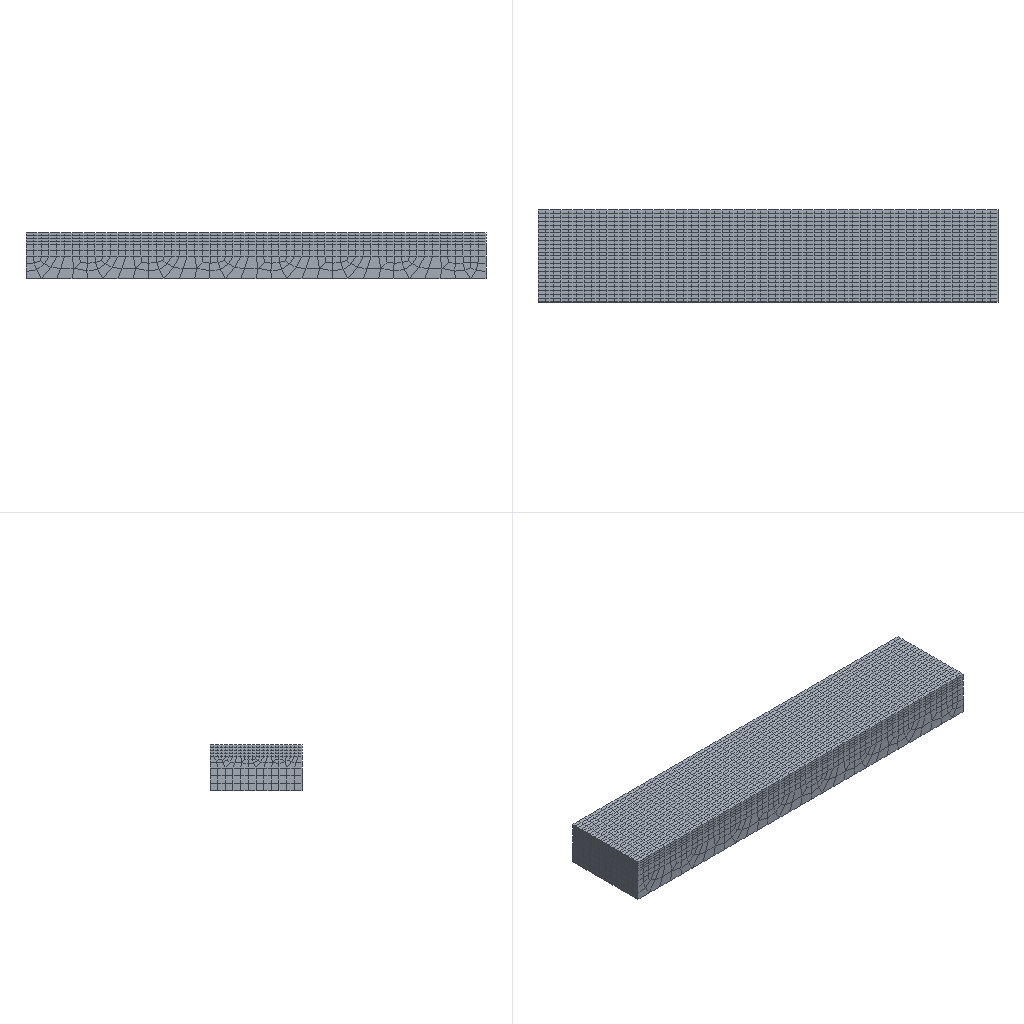Simulation study | abaqus
Set-up summary:
category,name,step,type,value,unit,region
solver,abaqus
solver,version,,,Abaqus/Explicit 2020
units,not stated in the deck,,not stated
analysis,deck,,transient,transient
load_step,Step-1,Step-1,transient
load_step,Step-2,Step-2,transient
load_step,requested,,,2
mesh,nodes,,,19787
mesh,elements,,,17886
element_type,C3D8,,solid,9996
element_type,R3D4,,rigid,7890
load,load commands in deck,,count,7
bc,support commands in deck,,count,36
material,MATERIAL-1,,in results
check,setup vs results,,match,"per instance, exact: element labels, types and connectivity; labels of the nodes the elements use; coordinates not compared"
Abaqus input file, long lists of numbers shortened:
*Heading
** Job name: Job-1 Model name: Model-3
** Generated by: Abaqus/CAE 2020
*Preprint, echo=NO, model=NO, history=NO, contact=NO
**
** PARTS
**
*Part, name=down
*Node
      1,   17.5,           0., 0.02419
      2,   17.5,          12., 0.02419
** (383 more lines like these left out)
*Element, type=R3D4
  1,   1,   7, 121,  68
  2,   7,   8, 122, 121
** (328 more lines like these left out)
*Node
    386, 1.07156592e-15,          12.,           0.
*Nset, nset=down-RefPt_, internal
386,
*Elset, elset=down, generate
   1,  330,    1
*End Part
**
*Part, name=plate
*Node
      1,          60.,          12.,          4.5
      2,           0.,          12.,          4.5
** (11628 more lines like these left out)
*Element, type=C3D8
   1,  310, 1081, 5131,  943,    1,   17,  589,  140
   2, 1081, 1082, 5132, 5131,   17,   18,  590,  589
** (9994 more lines like these left out)
*Nset, nset=_PickedSet2, internal, generate
     1,  11630,      1
*Elset, elset=_PickedSet2, internal, generate
    1,  9996,     1
** Section: Section-1
*Solid Section, elset=_PickedSet2, material=Material-1
,
*End Part
**
*Part, name=up1mm
*Node
      1,           0.,           0.,        -16.5
      2,           0.,           1.,        -17.5
** (7768 more lines like these left out)
*Element, type=R3D4
  1,   65, 2731, 2735,   64
  2, 2731, 2732, 2736, 2735
** (7558 more lines like these left out)
*Node
   7771, 1.01033359e-15,          12.,           0.
*Nset, nset=up1mm-RefPt_, internal
7771,
*Elset, elset=up1mm, generate
    1,  7560,     1
*End Part
**
**
** ASSEMBLY
**
*Assembly, name=Assembly
**
*Instance, name=down-1, part=down
*End Instance
**
*Instance, name=plate-1, part=plate
        -10.,           0.,         17.5
*End Instance
**
*Instance, name=up1mm-1, part=up1mm
          0.,           0.,          41.
*End Instance
**
*Nset, nset=blank, instance=plate-1, generate
     1,  11630,      1
*Elset, elset=blank, instance=plate-1, generate
    1,  9996,     1
*Nset, nset=_PickedSet19, internal, instance=down-1
 386,
*Nset, nset=_PickedSet20, internal, instance=up1mm-1
 7771,
*Nset, nset=_PickedSet25, internal, instance=up1mm-1
 7771,
*Nset, nset=_PickedSet36, internal, instance=plate-1
    2,    3,    5,    6,    9,   10,   13,   16,   76,   77,   78,  200,  201,  202,  311,  312
  313,  314,  315,  316,  317,  318,  319,  320,  321,  322,  323,  324,  325,  326,  327,  328
** (11 more lines like these left out)
*Elset, elset=_PickedSet36, internal, instance=plate-1
   60,  120,  180,  240,  300,  360,  420,  480,  540,  600,  660,  720,  780,  840,  900,  960
 1020, 1080, 1140, 1200, 1260, 1320, 1380, 1440, 1500, 1560, 1620, 1680, 1740, 1800, 1860, 1920
** (10 more lines like these left out)
*Nset, nset=_PickedSet37, internal, instance=plate-1
    2,    3,    5,    6,    9,   10,   13,   16,   76,   77,   78,  200,  201,  202,  311,  312
  313,  314,  315,  316,  317,  318,  319,  320,  321,  322,  323,  324,  325,  326,  327,  328
** (11 more lines like these left out)
*Elset, elset=_PickedSet37, internal, instance=plate-1
   60,  120,  180,  240,  300,  360,  420,  480,  540,  600,  660,  720,  780,  840,  900,  960
 1020, 1080, 1140, 1200, 1260, 1320, 1380, 1440, 1500, 1560, 1620, 1680, 1740, 1800, 1860, 1920
** (10 more lines like these left out)
*Nset, nset=_PickedSet38, internal, instance=up1mm-1
 7771,
*Nset, nset=_PickedSet40, internal, instance=up1mm-1
 7771,
*Elset, elset=__PickedSurf14_SPOS, internal, instance=up1mm-1, generate
    1,  7560,     1
*Surface, type=ELEMENT, name=_PickedSurf14, internal
__PickedSurf14_SPOS, SPOS
*Elset, elset=__PickedSurf15_S5, internal, instance=plate-1
  181,  182,  183,  184,  185,  186,  187,  188,  189,  190,  191,  192,  193,  194,  195,  196
  197,  198,  199,  200,  201,  202,  203,  204,  205,  206,  207,  208,  209,  210,  211,  212
** (88 more lines like these left out)
*Surface, type=ELEMENT, name=_PickedSurf15, internal
__PickedSurf15_S5, S5
*Elset, elset=__PickedSurf16_SPOS, internal, instance=down-1, generate
   1,  330,    1
*Surface, type=ELEMENT, name=_PickedSurf16, internal
__PickedSurf16_SPOS, SPOS
*Elset, elset=__PickedSurf17_S5, internal, instance=plate-1
 8583, 8595, 8631, 8633, 8706, 8718, 8754, 8756, 8829, 8841, 8877, 8879, 8952, 8964, 9000, 9002
 9075, 9087, 9123, 9125, 9198, 9210, 9246, 9248, 9321, 9333, 9369, 9371, 9444, 9456, 9492, 9494
** (1 more lines like these left out)
*Elset, elset=__PickedSurf17_S6, internal, instance=plate-1
 8584, 8587, 8590, 8593, 8596, 8599, 8602, 8605, 8636, 8637, 8638, 8707, 8710, 8713, 8716, 8719
 8722, 8725, 8728, 8759, 8760, 8761, 8830, 8833, 8836, 8839, 8842, 8845, 8848, 8851, 8882, 8883
** (7 more lines like these left out)
*Elset, elset=__PickedSurf17_S3, internal, instance=plate-1
 8589, 8601, 8607, 8610, 8612, 8615, 8619, 8623, 8626, 8629, 8635, 8712, 8724, 8730, 8733, 8735
 8738, 8742, 8746, 8749, 8752, 8758, 8835, 8847, 8853, 8856, 8858, 8861, 8865, 8869, 8872, 8875
** (7 more lines like these left out)
*Elset, elset=__PickedSurf17_S4, internal, instance=plate-1
 8616, 8620, 8624, 8628, 8739, 8743, 8747, 8751, 8862, 8866, 8870, 8874, 8985, 8989, 8993, 8997
 9108, 9112, 9116, 9120, 9231, 9235, 9239, 9243, 9354, 9358, 9362, 9366, 9477, 9481, 9485, 9489
** (1 more lines like these left out)
*Surface, type=ELEMENT, name=_PickedSurf17, internal
__PickedSurf17_S5, S5
__PickedSurf17_S6, S6
__PickedSurf17_S4, S4
__PickedSurf17_S3, S3
*Rigid Body, ref node=down-1.down-RefPt_, elset=down-1.down
*Rigid Body, ref node=up1mm-1.up1mm-RefPt_, elset=up1mm-1.up1mm
*Element, type=MASS, elset=_PickedSet39_Inertia-1_MASS_
1, down-1.386
2, up1mm-1.777
*Mass, elset=_PickedSet39_Inertia-1_MASS_
0.1,
*Element, type=ROTARYI, elset=_PickedSet39_Inertia-1_ROTI_
3, down-1.386
4, up1mm-1.777
*Rotary Inertia, elset=_PickedSet39_Inertia-1_ROTI_
0.1, 0.1, 0.1, 0., 0., 0.
*End Assembly
*Amplitude, name=Amp-1
             0.,              0.,              1.,              1.
*Amplitude, name=ultrasound, definition=PERIODIC
1,         125664.,              0.,              0.
             0.,              1.
**
** MATERIALS
**
*Material, name=Material-1
*Density
 2.7e-09,
*Elastic
71700., 0.33
*Plastic
 222.411,  0.
    270., 0.1
    300., 0.3
**
** INTERACTION PROPERTIES
**
*Surface Interaction, name=IntProp-1
*Friction
 0.3,
*Surface Behavior, pressure-overclosure=HARD
**
** BOUNDARY CONDITIONS
**
** Name: BC-1 Type: 位移/转角
*Boundary
_PickedSet19, 1, 1
_PickedSet19, 2, 2
_PickedSet19, 3, 3
_PickedSet19, 4, 4
_PickedSet19, 5, 5
_PickedSet19, 6, 6
**
** PREDEFINED FIELDS
**
** Name: Predefined Field-1   Type: Velocity
*Initial Conditions, type=VELOCITY
_PickedSet25, 1, 0.
_PickedSet25, 2, 0.
_PickedSet25, 3, -30.
** Name: Predefined Field-2   Type: Velocity
*Initial Conditions, type=VELOCITY
_PickedSet37, 1, -17.
_PickedSet37, 2, 0.
_PickedSet37, 3, 0.
**
** INTERACTIONS
**
** Interaction: Int-3
*Contact, op=NEW
*Contact Inclusions, ALL EXTERIOR
*Contact Property Assignment
 ,  , IntProp-1
** ----------------------------------------------------------------
**
** STEP: Step-1
**
*Step, name=Step-1, nlgeom=YES
*Dynamic, Explicit
, 1.
*Bulk Viscosity
0.06, 1.2
** Mass Scaling: Semi-Automatic
**               Whole Model
*Fixed Mass Scaling, dt=1e-07, type=below min, factor=5000.
**
** BOUNDARY CONDITIONS
**
** Name: BC-1 Type: 位移/转角
*Boundary, op=NEW
_PickedSet19, 1, 1
_PickedSet19, 2, 2
_PickedSet19, 3, 3
_PickedSet19, 4, 4
_PickedSet19, 5, 5
_PickedSet19, 6, 6
** Name: BC-2 Type: 位移/转角
*Boundary, op=NEW, amplitude=Amp-1
_PickedSet20, 1, 1
_PickedSet20, 2, 2
_PickedSet20, 3, 3, -0.7
_PickedSet20, 4, 4
_PickedSet20, 5, 5
_PickedSet20, 6, 6
**
** INTERACTIONS
**
** Interaction: Int-1
*Contact Pair, interaction=IntProp-1, mechanical constraint=PENALTY, cpset=Int-1
_PickedSurf14, _PickedSurf15
** Interaction: Int-2
*Contact Pair, interaction=IntProp-1, mechanical constraint=PENALTY, cpset=Int-2
_PickedSurf16, _PickedSurf17
**
** OUTPUT REQUESTS
**
*Restart, write, number interval=1, time marks=NO
**
** FIELD OUTPUT: F-Output-1
**
*Output, field, number interval=100
*Node Output
RF, U
*Element Output, directions=YES
PEEQ, S
*Contact Output
CSTRESS,
**
** HISTORY OUTPUT: H-Output-1
**
*Output, history
*Energy Output
ALLIE, ALLKE
*End Step
** ----------------------------------------------------------------
**
** STEP: Step-2
**
*Step, name=Step-2, nlgeom=YES
*Dynamic, Explicit
, 1.
*Bulk Viscosity
0.06, 1.2
** Mass Scaling: Semi-Automatic
**               blank
*Fixed Mass Scaling, elset=blank, factor=5000.
**
** BOUNDARY CONDITIONS
**
** Name: BC-1 Type: 位移/转角
*Boundary, op=NEW, amplitude=Amp-1
_PickedSet19, 1, 1
_PickedSet19, 2, 2
_PickedSet19, 3, 3
_PickedSet19, 4, 4
_PickedSet19, 5, 5, -1.
_PickedSet19, 6, 6
** Name: BC-2 Type: 位移/转角
*Boundary, op=NEW
** Name: BC-3 Type: 位移/转角
*Boundary, op=NEW, amplitude=Amp-1
_PickedSet36, 1, 1, -17.5
_PickedSet36, 2, 2
_PickedSet36, 3, 3
_PickedSet36, 4, 4
_PickedSet36, 5, 5
_PickedSet36, 6, 6
** Name: BC-6 Type: 位移/转角
*Boundary, op=NEW, amplitude=ultrasound
_PickedSet38, 1, 1
_PickedSet38, 2, 2
_PickedSet38, 3, 3, 0.075
_PickedSet38, 4, 4
_PickedSet38, 6, 6
** Name: BC-7 Type: 位移/转角
*Boundary, op=NEW, amplitude=Amp-1
_PickedSet40, 5, 5, 1.
**
** OUTPUT REQUESTS
**
*Restart, write, number interval=1, time marks=NO
**
** FIELD OUTPUT: F-Output-1
**
*Output, field, number interval=100
*Node Output
RF, U, V
*Element Output, directions=YES
E, MISES, PEEQ, S
*Contact Output
CSTRESS,
**
** HISTORY OUTPUT: H-Output-1
**
*Output, history
*Energy Output
ALLIE, ALLKE
*End Step
Results summary:
result,step,Step-1,completed,increments=331296 time=1.0/1.0
result,step,Step-2,partial,increments=66072 time=0.1231/1.0
result,analysis,,,transient
result,last_loadstep,,,2
result,primary field,,,U
result,reaction total,,FX,682596825.357,model units
result,reaction total,,FY,424995765.246,model units
result,reaction total,,FZ,560580463302.733,model units